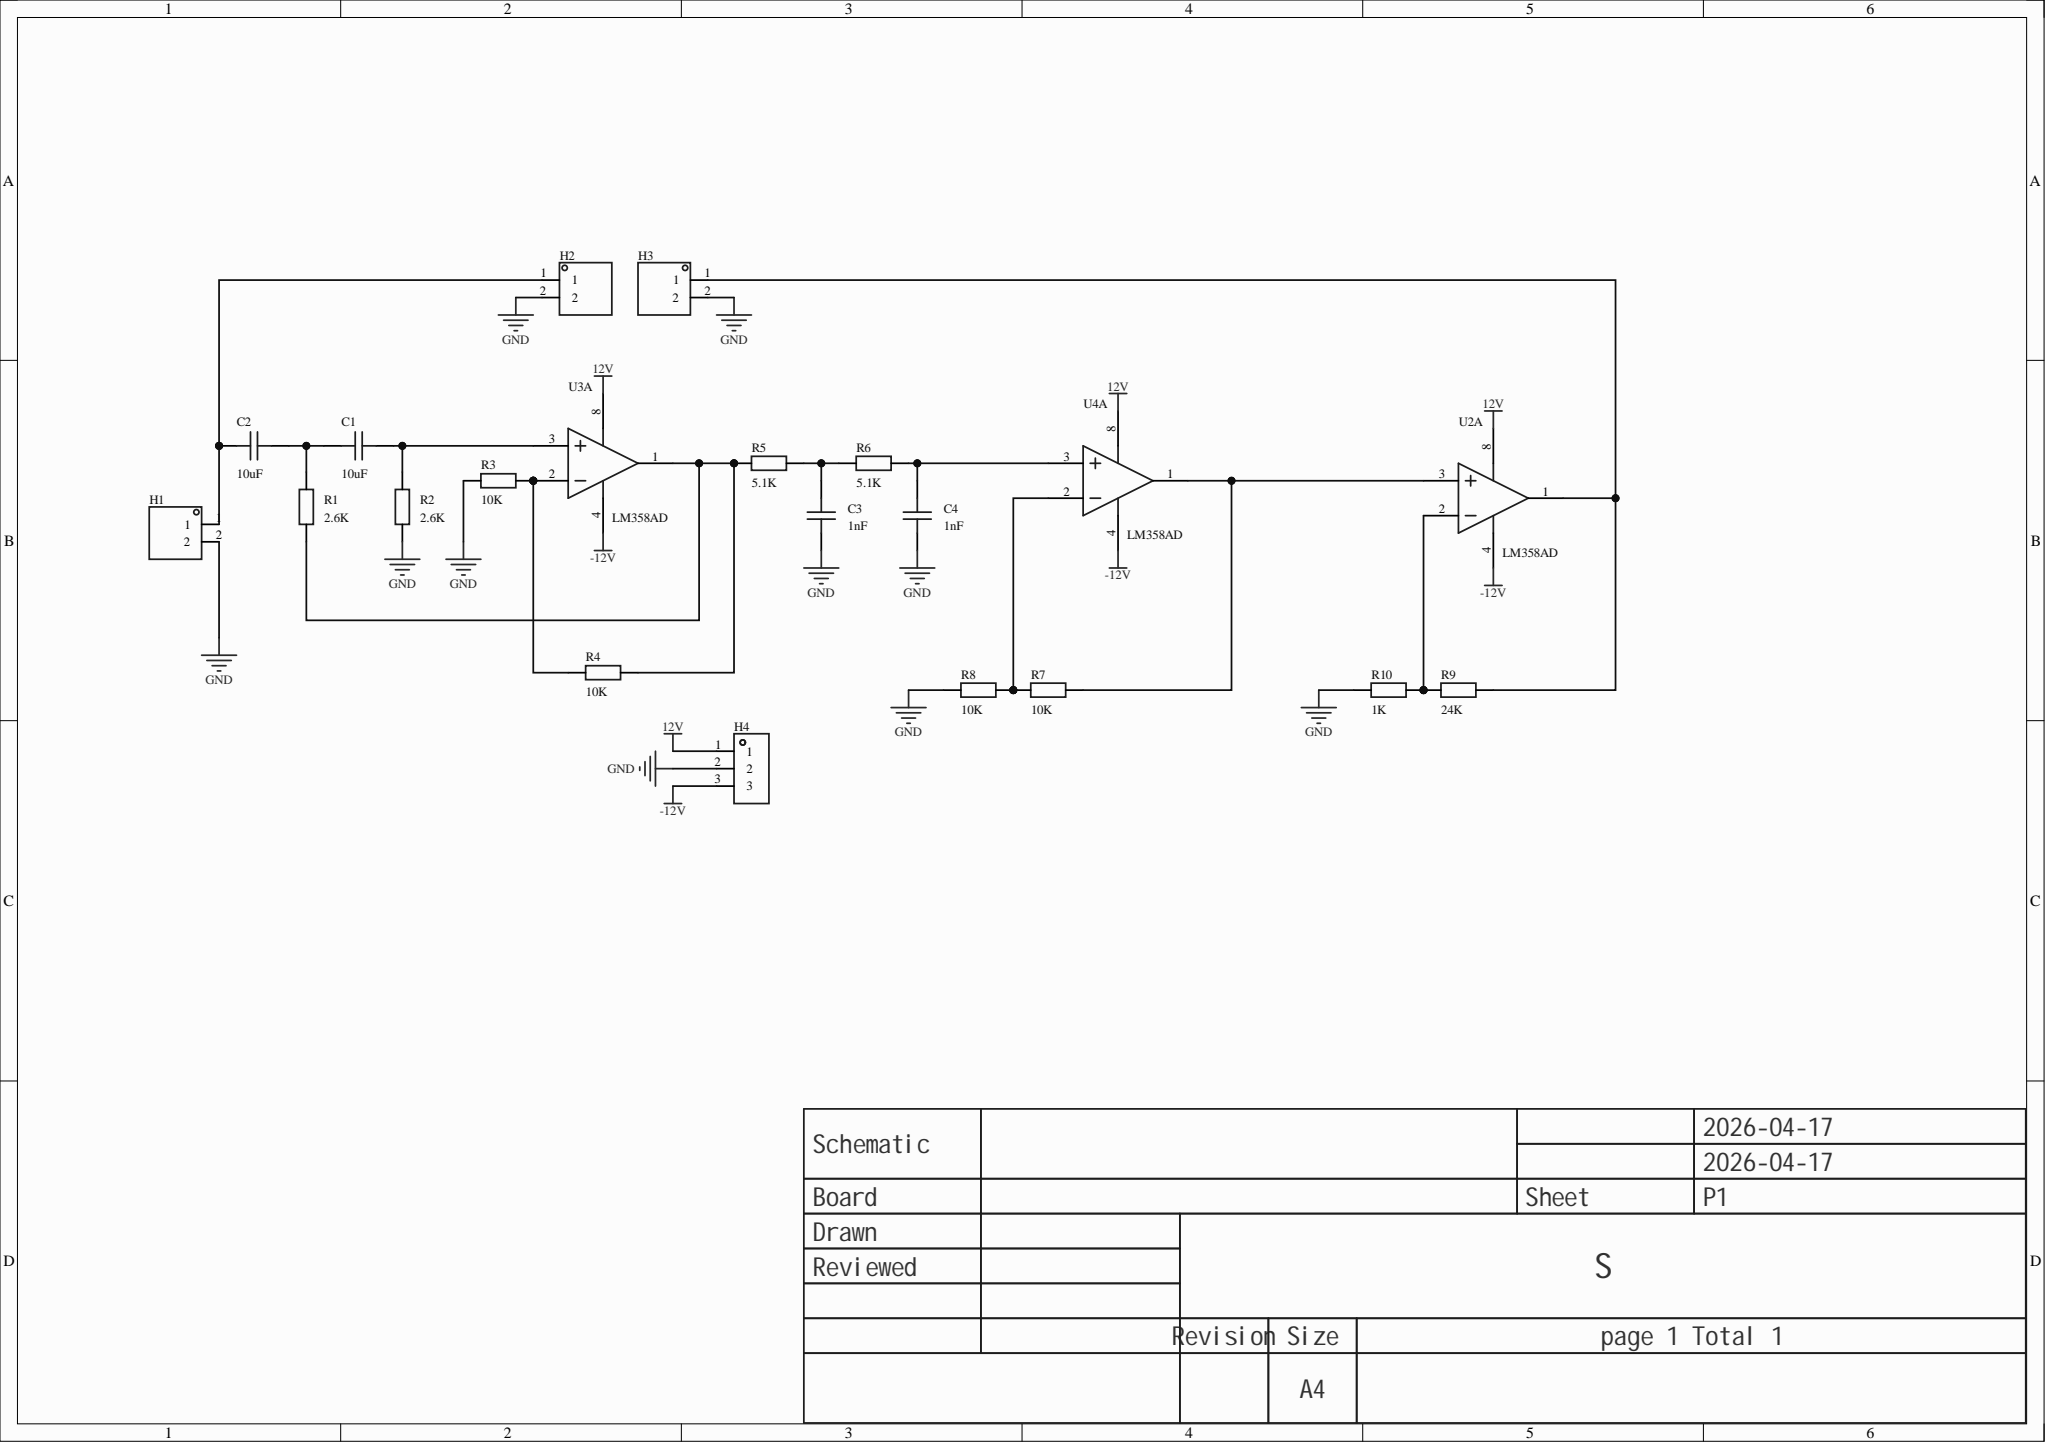Circuit board | Altium Designer | 21 parts | 14 nets
Bill of materials:
Comment,Description,Designator,Footprint,LibRef,Quantity
"10uF","","C1, C2","C0805","CAP_0805","2"
"1nF","","C3, C4","C0805","CAP_0805","2"
"","","H1, H2, H3","HDR-TH_2P-P2.54-V-M-1","HDR-M_2.54_1x2P","3"
"","","H4","HDR-TH_3P-P2.54-V-M","HDR-M_2.54_1x3P","1"
"2.6K","","R1, R2","R0805","Res_0805","2"
"10K","","R3, R4, R7, R8","R0805","Res_0805","4"
"5.1K","","R5, R6","R0805","Res_0805","2"
"24K","","R9","R0805","Res_0805","1"
"1K","","R10","R0805","Res_0805","1"
"LM358AD","Amplifier count: 2; Rail-to-rail: -; Gain bandwidth product (GBW): -; Input offset voltage (Vos): -; Slew rate (SR): -; Input bias current (Ib): -;","U2, U3, U4","PDIP-8_L9.5-W6.4-P2.54-LS7.6-BL","CA3240-DIP-8","3"
Netlist (Protel format):
[
C1
C0805
10uF



]
[
C2
C0805
10uF



]
[
C3
C0805
1nF



]
[
C4
C0805
1nF



]
[
H1
HDR-TH_2P-P2.54-V-M-1




]
[
H2
HDR-TH_2P-P2.54-V-M-1




]
[
H3
HDR-TH_2P-P2.54-V-M-1




]
[
H4
HDR-TH_3P-P2.54-V-M




]
[
R1
R0805
2.6K



]
[
R2
R0805
2.6K



]
[
R3
R0805
10K



]
[
R4
R0805
10K



]
[
R5
R0805
5.1K



]
[
R6
R0805
5.1K



]
[
R7
R0805
10K



]
[
R8
R0805
10K



]
[
R9
R0805
24K



]
[
R10
R0805
1K



]
[
U2
PDIP-8_L9.5-W6.4-P2.54-LS7.6-BL
LM358AD



]
[
U3
PDIP-8_L9.5-W6.4-P2.54-LS7.6-BL
LM358AD



]
[
U4
PDIP-8_L9.5-W6.4-P2.54-LS7.6-BL
LM358AD



]
(
NetR9_1
R9-1
R10-2
U2-2
)
(
NetR7_2
R7-2
U2-3
U4-1
)
(
NetR7_1
R7-1
R8-2
U4-2
)
(
NetR3_2
R3-2
R4-1
U3-2
)
(
NetR1_1
R1-1
R4-2
R5-1
U3-1
)
(
NetH3_1
H3-1
R9-2
U2-1
)
(
NetC4_2
C4-2
R6-2
U4-3
)
(
NetC3_2
C3-2
R5-2
R6-1
)
(
NetC2_1
C2-1
H1-1
H2-1
)
(
NetC1_2
C1-2
R2-2
U3-3
)
(
NetC1_1
C1-1
C2-2
R1-2
)
(
GND
C3-1
C4-1
H1-2
H2-2
H3-2
H4-2
R2-1
R3-1
R8-1
R10-1
)
(
-12V
H4-3
U2-4
U3-4
U4-4
)
(
12V
H4-1
U2-8
U3-8
U4-8
)